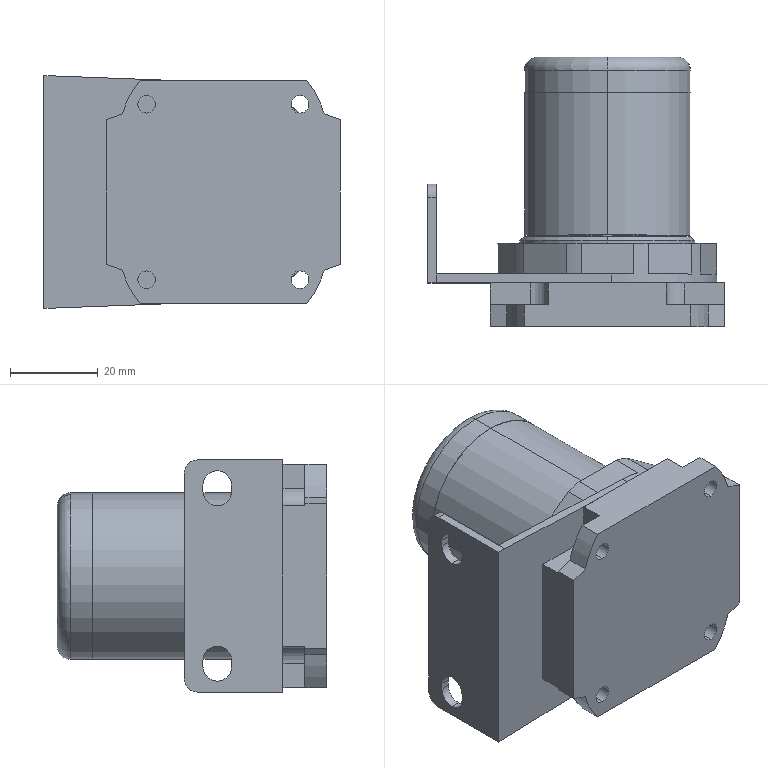Part | NX | features BREP 1 | 1 solid | 100 faces | box 67.7 x 61.5 x 53 mm | volume 93011 mm3 | plane 58 | cylinder 38 | torus 2 | cone 2 | commonest cylinder face diameters 4 x8 6.5 x6 40 x6 50 x6 8 x4 6 x2